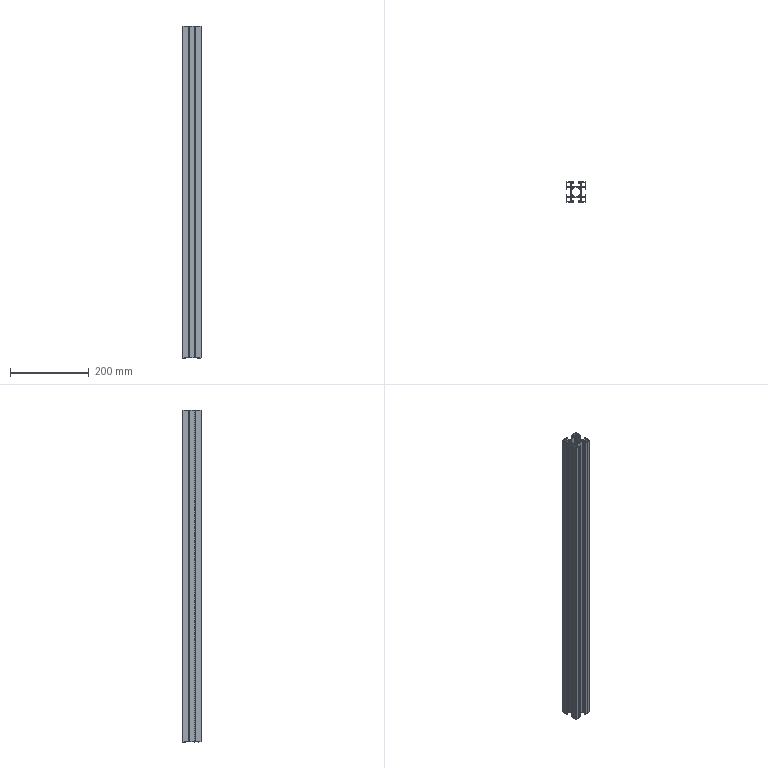Part | STEP file | 46A-00006CC11-845mm | 1 solid | 142 faces | box 50 x 50 x 845 mm | volume 496431 mm3 | cylinder 84 | plane 58 | commonest cylinder face diameters 1 x24 4 x24 1.5 x16 3.7 x8 6.7 x8 2 x4